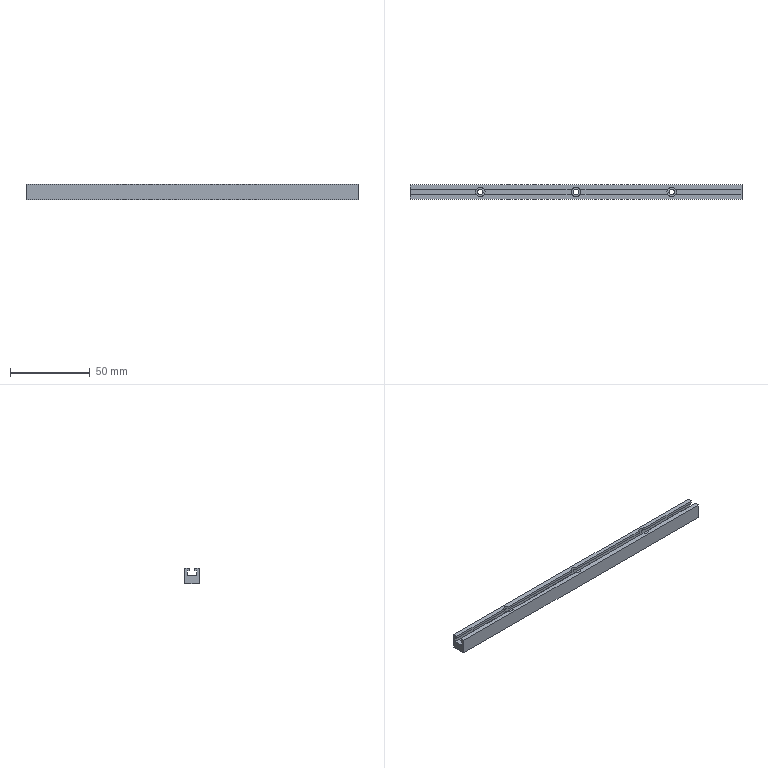Part | STEP file | QA-SENAT33H_208_V44_W104_X164_N3_5 | 1 solid | 50 faces | box 208 x 9 x 9.5 mm | volume 12749 mm3 | plane 38 | cylinder 12 | commonest cylinder face diameters 3.5 x6 6 x6